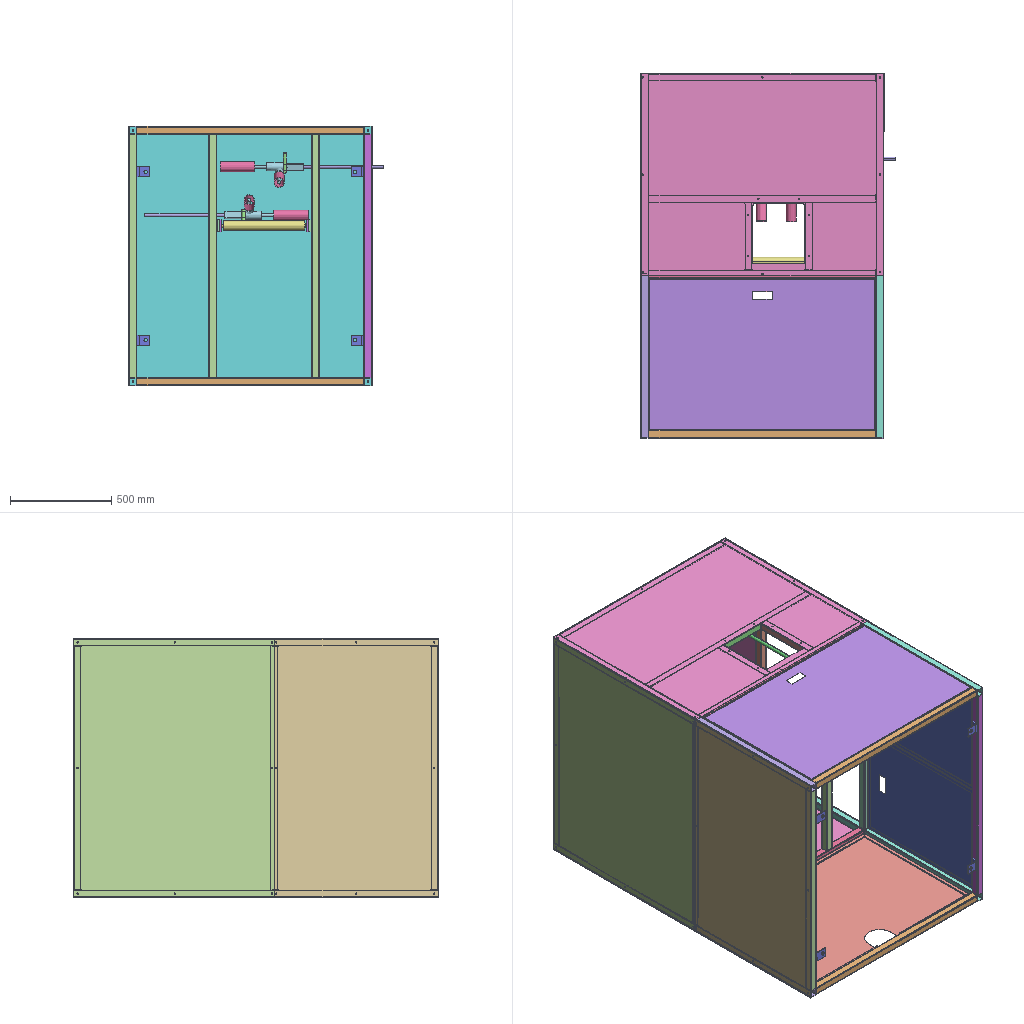Assembly | SolidWorks | 25 different items | 45 placed | box 1258 x 1804 x 1282 mm
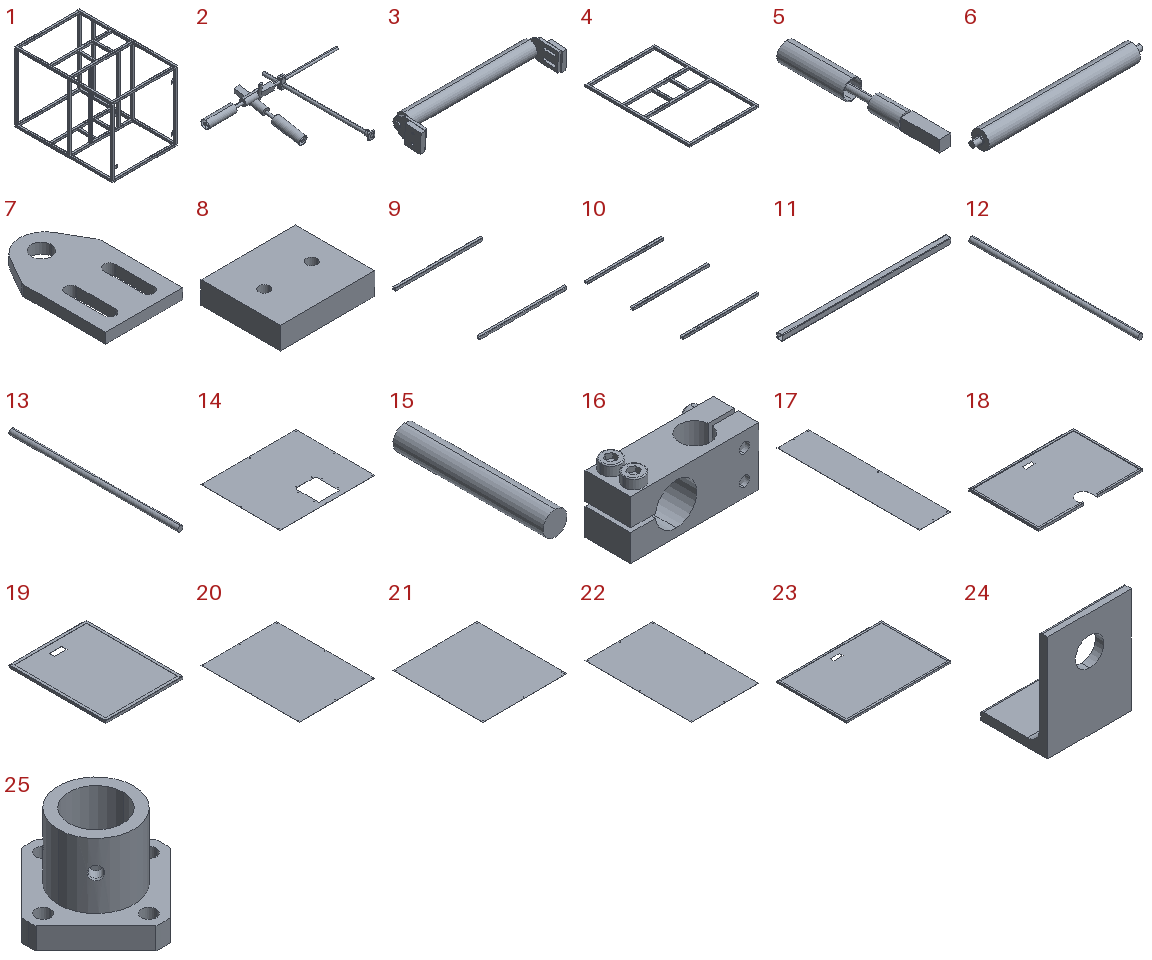Parts list (item | name | quantity | parent item | size | volume | features):
1 | (subassembly) | x1 | - | 1200 x 1802 x 1280 mm | 10178474 mm3 | features ReferencePattern 2, AEMSimFeature 1, LocalLPattern 1
2 | (subassembly) | x2 | - | 805 x 660 x 172.187 mm | 944058 mm3 | features AEMSimFeature 1
3 | (subassembly) | x1 | - | 464 x 110.124 x 63.961 mm | 853644 mm3 | features AEMSimFeature 1
4 | - | x2 | in 1 | 1200 x 1800 x 40 mm | 3242202 mm3 | features WeldCornerFeat 1, WeldMemberFeat 1, WeldmentFeature 1
5 | - | x4 | in 2 | 50 x 410 x 50 mm | 288046 mm3 | features ICE 3, Extrusion 1
6 | - | x1 | in 3 | 445 x 47 x 47 mm | 702617 mm3 | features Revolution 1
7 | - | x2 | in 3 | 60 x 96.962 x 8 mm | 34530 mm3 | features ICE 2, Extrusion 1, Fillet 1
8 | - | x2 | in 3 | 60 x 50 x 14 mm | 40983 mm3 | features Extrusion 1, HoleWzd 1
9 | - | x1 | in 1 | 1200 x 1200 x 40 mm | 799721 mm3 | features WeldMemberFeat 1, WeldmentFeature 1
10 | - | x1 | in 1 | 1200 x 1550 x 40 mm | 1199581 mm3 | features WeldMemberFeat 1, WeldmentFeature 1
11 | - | x4 | in 1 | 1200 x 40 x 40 mm | 399860 mm3 | features WeldMemberFeat 1, WeldmentFeature 1
12 | - | x2 | in 2 | 20 x 660 x 20 mm | 207345 mm3 | features Extrusion 1
13 | - | x2 | in 2 | 16 x 495 x 16 mm | 99236 mm3 | features Extrusion 1, ICE 1
14 | - | x2 | - | 1200 x 1000 x 1.2 mm | 1346035 mm3 | features Fillet 3, HoleWzd 2, FlatPattern 1, ICE 1, SMBaseFlange 1, SheetMetal 1
15 | - | x2 | in 2 | 16 x 100 x 16 mm | 19399 mm3 | features Extrusion 1, ICE 1
16 | - | x2 | in 2 | 62 x 26.8 x 32.8 mm | 26392 mm3 | features ICE 7, Fillet 2, MirrorSolid 2, MoveCopyBody 2, Revolution 2, Extrusion 1
17 | - | x1 | - | 285 x 1280 x 1.2 mm | 437432 mm3 | features FlatPattern 1, HoleWzd 1, SMBaseFlange 1, SheetMetal 1
18 | - | x1 | - | 1116 x 747 x 25 mm | 1145204 mm3 | features EdgeFlange 2, ICE 2, FlatPattern 1, SMBaseFlange 1, SheetMetal 1
19 | - | x2 | - | 597 x 747 x 20 mm | 645008 mm3 | features EdgeFlange 2, FlatPattern 1, ICE 1, SMBaseFlange 1, SheetMetal 1
20 | - | x1 | - | 990 x 1280 x 1.2 mm | 1520312 mm3 | features FlatPattern 1, HoleWzd 1, SMBaseFlange 1, SheetMetal 1
21 | - | x1 | - | 1200 x 1280 x 1.2 mm | 1842780 mm3 | features Fillet 2, HoleWzd 2, FlatPattern 1, SMBaseFlange 1, SheetMetal 1
22 | - | x1 | - | 810 x 1280 x 1.2 mm | 1243832 mm3 | features FlatPattern 1, HoleWzd 1, SMBaseFlange 1, SheetMetal 1
23 | - | x1 | - | 1116 x 747 x 20 mm | 1155364 mm3 | features EdgeFlange 2, FlatPattern 1, ICE 1, SMBaseFlange 1, SheetMetal 1
24 | - | x4 | in 1 | 50 x 40 x 63 mm | 23831 mm3 | features ICE 1, WeldMemberFeat 1, WeldmentFeature 1
25 | - | x2 | in 2 | 50 x 50 x 32 mm | 15595 mm3 | features BaseBody 1
Mates (type | each side: item.copy, entity, surface, feature):
In the top assembly
Coincident | 14.1 face plane Base-Flange1 | 14.2 face plane Base-Flange1 | 2 times
Coincident | 4.1 face | assembly face | 3 times
Coincident | assembly face | 21.1 face plane Base-Flange1 | 2 times
Coincident | 14.2 face plane Base-Flange1 | 21.1 face plane Base-Flange1
Coincident | assembly face | 22.1 face plane Base-Flange1 | 3 times
Coincident | 4.2 face plane Square Tube 40 X 40 X 2.3(1) | assembly face | 2 times
Coincident | assembly face | assembly face | 2 times
DistanceDim | assembly face | assembly face
Coincident | 11.1 face plane Square Tube 40 X 40 X 2.3(1) | 25.1 face plane Input1 | 2 times
DistanceDim | 25.1 face plane Input1 | 4.2 face plane Square Tube 40 X 40 X 2.3(1)
Coincident | 11.2 face plane Square Tube 40 X 40 X 2.3(1) | 25.2 face plane Input1 | 2 times
DistanceDim | 25.2 face plane Input1 | 25.1 face plane Input1
Coincident | 4.1 face plane Square Tube 40 X 40 X 2.3(1) | 14.2 face plane Base-Flange1
Coincident | 4.1 face plane Square Tube 40 X 40 X 2.3(1) | assembly face | 3 times
Coincident | 9.1 face plane Square Tube 40 X 40 X 2.3(1) | 21.1 face plane Base-Flange1 | 2 times
Coincident | 9.1 face plane Square Tube 40 X 40 X 2.3(1) | 22.1 face plane Base-Flange1
Coincident | 9.1 face plane Square Tube 40 X 40 X 2.3(1) | assembly face
Width | 6.1 face plane Revolve1 | 6.1 face plane Revolve1 | 11.2 face plane Square Tube 40 X 40 X 2.3(1) | 11.1 face plane Square Tube 40 X 40 X 2.3(1)
Coincident | 11.2 face plane Square Tube 40 X 40 X 2.3(1) | 7.1 face plane Boss-Extrude1
DistanceDim | 4.2 face plane Square Tube 40 X 40 X 2.3(1) | 8.1 face plane Boss-Extrude1
DistanceDim | assembly face | 4.2 face
Coincident | 4.2 face | assembly face
DistanceDim | assembly face | 4.2 face plane Square Tube 40 X 40 X 2.3(1) | 2 times
Coincident | 10.1 face plane Square Tube 40 X 40 X 2.3(1) | assembly face | 5 times
DistanceDim | assembly face | 4.1 face plane Square Tube 40 X 40 X 2.3(1) | 2 times
DistanceDim | assembly face | 10.1 face plane Square Tube 40 X 40 X 2.3(1)
DistanceDim | assembly face | 11.3 face plane Square Tube 40 X 40 X 2.3(1)
Coincident | 4.2 face plane Square Tube 40 X 40 X 2.3(1) | 23.1 face plane Base-Flange1
Coincident | 4.2 face plane Square Tube 40 X 40 X 2.3(1) | 23.1 face plane Edge-Flange1
Coincident | 4.1 face plane Square Tube 40 X 40 X 2.3(1) | 18.1 face plane Edge-Flange1
Coincident | 4.1 face plane Square Tube 40 X 40 X 2.3(1) | 18.1 face plane Base-Flange1
DistanceDim | 18.1 face plane Edge-Flange1 | 4.1 face plane Square Tube 40 X 40 X 2.3(1)
Coincident | 10.1 face plane Square Tube 40 X 40 X 2.3(1) | 19.1 face plane Edge-Flange1
Coincident | 10.1 face plane Square Tube 40 X 40 X 2.3(1) | 19.1 face plane Base-Flange1
DistanceDim | 19.1 face plane Edge-Flange1 | 4.2 face plane Square Tube 40 X 40 X 2.3(1)
DistanceDim | assembly face | 10.1 face | 2 times
Coincident | 14.2 face plane Base-Flange1 | assembly face
Coincident | assembly face | 20.1 face plane Base-Flange1 | 2 times
Coincident | assembly edge | 20.1 face plane Base-Flange1
Coincident | 21.1 face plane Base-Flange1 | assembly face
Coincident | 4.2 face plane Square Tube 40 X 40 X 2.3(1) | 14.1 face plane Base-Flange1 | 3 times
DistanceDim | 23.1 face plane Edge-Flange1 | 4.2 face plane Square Tube 40 X 40 X 2.3(1)
Coincident | 4.1 face plane Square Tube 40 X 40 X 2.3(1) | 20.1 face plane Base-Flange1 | 2 times
Coincident | 11.3 face plane Square Tube 40 X 40 X 2.3(1) | 22.1 face plane Base-Flange1
Coincident | 4.2 face plane Square Tube 40 X 40 X 2.3(1) | 22.1 face plane Base-Flange1
Coincident | 22.1 face plane Base-Flange1 | 20.1 face plane Base-Flange1
Coincident | 9.1 face plane Square Tube 40 X 40 X 2.3(1) | 17.1 face plane Base-Flange1
Coincident | 21.1 face plane Base-Flange1 | 17.1 face plane Base-Flange1
Coincident | 14.1 face plane Base-Flange1 | 17.1 face plane Base-Flange1
Coincident | 19.1 face plane Base-Flange1 | 19.2 face plane Base-Flange1
DistanceDim | 19.2 face plane Edge-Flange1 | 4.1 face plane Square Tube 40 X 40 X 2.3(1)
Coincident | 10.1 face plane Square Tube 40 X 40 X 2.3(1) | 19.2 face plane Edge-Flange1
In subassembly 2
Concentric | 12.1 face cylinder Boss-Extrude1 | 25.3 face cylinder Input1
Coincident | 12.1 face plane Boss-Extrude1 | 25.3 face plane Input1
Concentric | 12.1 face cylinder Boss-Extrude1 | 16.1 face cylinder Cut-Extrude1
Concentric | 16.1 face cylinder Boss-Extrude1 | 13.1 face cylinder Boss-Extrude1
Parallel | 12.1 plane | 25.3 face plane Input1
DistanceDim | 16.1 face plane Boss-Extrude1 | 13.1 face plane Boss-Extrude1
DistanceDim | 16.1 face plane Boss-Extrude1 | 12.1 face plane Boss-Extrude1
Coincident | 13.1 face plane Cut-Extrude1 | 15.1 face plane Cut-Extrude1
Tangent | 13.1 face cylinder Boss-Extrude1 | 15.1 face plane Cut-Extrude1
PlanarAngleDim | 25.3 face plane Input1 | 15.1 face plane Cut-Extrude1
Tangent | 13.1 face plane Boss-Extrude1 | 15.1 face cylinder Boss-Extrude1
Parallel | 25.3 face plane Input1 | 16.1 face plane Boss-Extrude1
Coincident | 13.1 face plane Boss-Extrude1 | 5.1 face plane Boss-Extrude3
Concentric | 13.1 face cylinder Boss-Extrude1 | 5.1 face cylinder Boss-Extrude4
Coincident | 13.1 face plane Cut-Extrude1 | 5.2 face plane Boss-Extrude3
Tangent | 13.1 face plane Boss-Extrude1 | 5.2 face cylinder Boss-Extrude4
In subassembly 3
Concentric | 6.2 face cylinder Revolve1 | 7.2 face cylinder Cut-Extrude1
DistanceDim | 6.2 face plane Revolve1 | 7.2 face plane Boss-Extrude1
Concentric | 6.2 face cylinder Revolve1 | 7.3 face cylinder Cut-Extrude1
DistanceDim | 7.3 face plane Boss-Extrude1 | 6.2 face plane Revolve1
Coincident | 7.2 face plane Boss-Extrude1 | 8.2 face plane Boss-Extrude1 | 2 times
DistanceDim | 8.2 face plane Boss-Extrude1 | 7.2 face plane Boss-Extrude1
Coincident | 7.3 face plane Boss-Extrude1 | 8.3 face plane Boss-Extrude1 | 2 times
Coincident | 8.2 face plane Boss-Extrude1 | 8.3 face plane Boss-Extrude1
In subassembly 1
Coincident | 4.3 face plane Square Tube 40 X 40 X 2.3(1) | 9.2 face plane Square Tube 40 X 40 X 2.3(1) | 3 times
Coincident | 4.4 face plane Square Tube 40 X 40 X 2.3(1) | 9.2 face plane Square Tube 40 X 40 X 2.3(1) | 3 times
Coincident | 4.3 face plane Square Tube 40 X 40 X 2.3(1) | 10.2 face plane Square Tube 40 X 40 X 2.3(1) | 2 times
Coincident | 4.4 face plane Square Tube 40 X 40 X 2.3(1) | 11.4 face plane Square Tube 40 X 40 X 2.3(1) | 2 times
DistanceDim | 10.2 face plane Square Tube 40 X 40 X 2.3(1) | 11.4 face plane Square Tube 40 X 40 X 2.3(1)
Coincident | 4.4 face plane Square Tube 40 X 40 X 2.3(1) | 11.5 face plane Square Tube 40 X 40 X 2.3(1)
Coincident | 11.4 face plane Square Tube 40 X 40 X 2.3(1) | 11.5 face plane Square Tube 40 X 40 X 2.3(1)
DistanceDim | 11.4 face plane Square Tube 40 X 40 X 2.3(1) | 11.5 face plane Square Tube 40 X 40 X 2.3(1)
Coincident | 4.3 face plane Square Tube 40 X 40 X 2.3(1) | 11.6 face plane Square Tube 40 X 40 X 2.3(1) | 3 times
Coincident | 11.5 face plane Square Tube 40 X 40 X 2.3(1) | 11.7 face plane Square Tube 40 X 40 X 2.3(1)
Coincident | 4.3 face plane Square Tube 40 X 40 X 2.3(1) | 11.7 face plane Square Tube 40 X 40 X 2.3(1) | 2 times
Coincident | 10.2 face plane Square Tube 40 X 40 X 2.3(1) | 24.1 face plane Unequal Angle 6.3-4-5(1) | 2 times
DistanceDim | 24.1 face plane Unequal Angle 6.3-4-5(1) | 4.3 face plane Square Tube 40 X 40 X 2.3(1)
Coincident | 24.2 face plane Unequal Angle 6.3-4-5(1) | 11.6 face plane Square Tube 40 X 40 X 2.3(1) | 2 times
Coincident | 24.2 face plane Unequal Angle 6.3-4-5(1) | 24.1 face plane Unequal Angle 6.3-4-5(1)